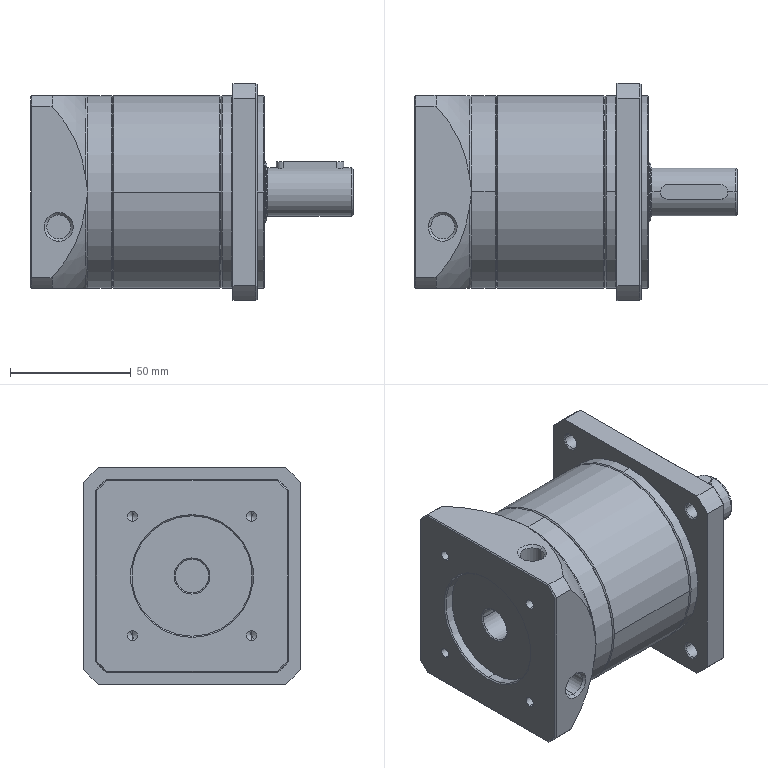Part | SolidWorks | features BaseBody 1 | 1 solid | 161 faces | box 134 x 90 x 90 mm | volume 530588 mm3 | cone 62 | cylinder 55 | plane 32 | spline 8 | sphere 4 | commonest cylinder face diameters 6.5 x10 4.2 x8 10 x8 80 x8 6 x5 107 x4